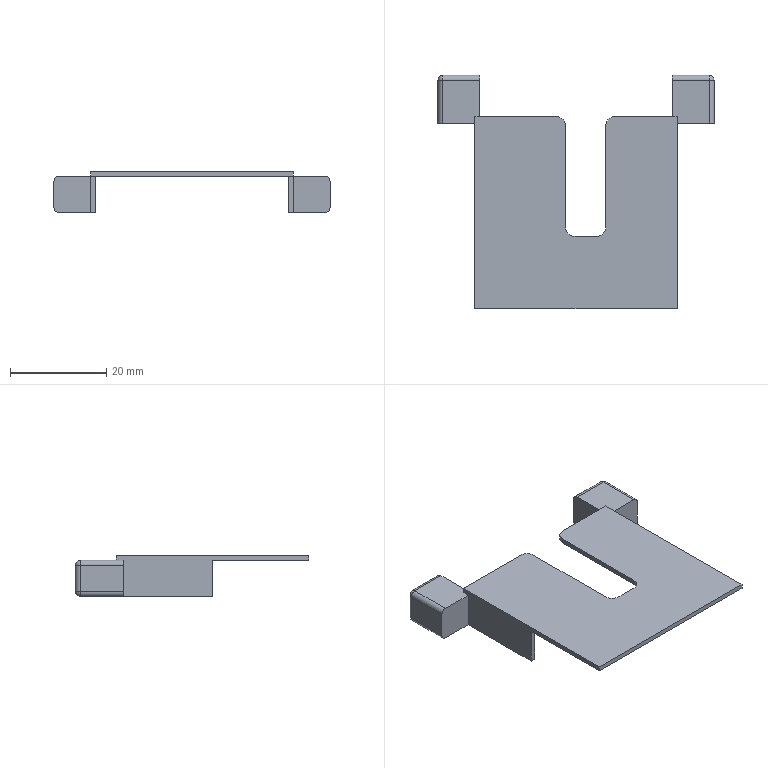Part | STEP file | ASND-0110-SDS_7 | 1 solid | 42 faces | box 57.4 x 48.5 x 8.5 mm | volume 3034 mm3 | plane 24 | cylinder 14 | sphere 4 | commonest cylinder face diameters 2 x10 4 x4